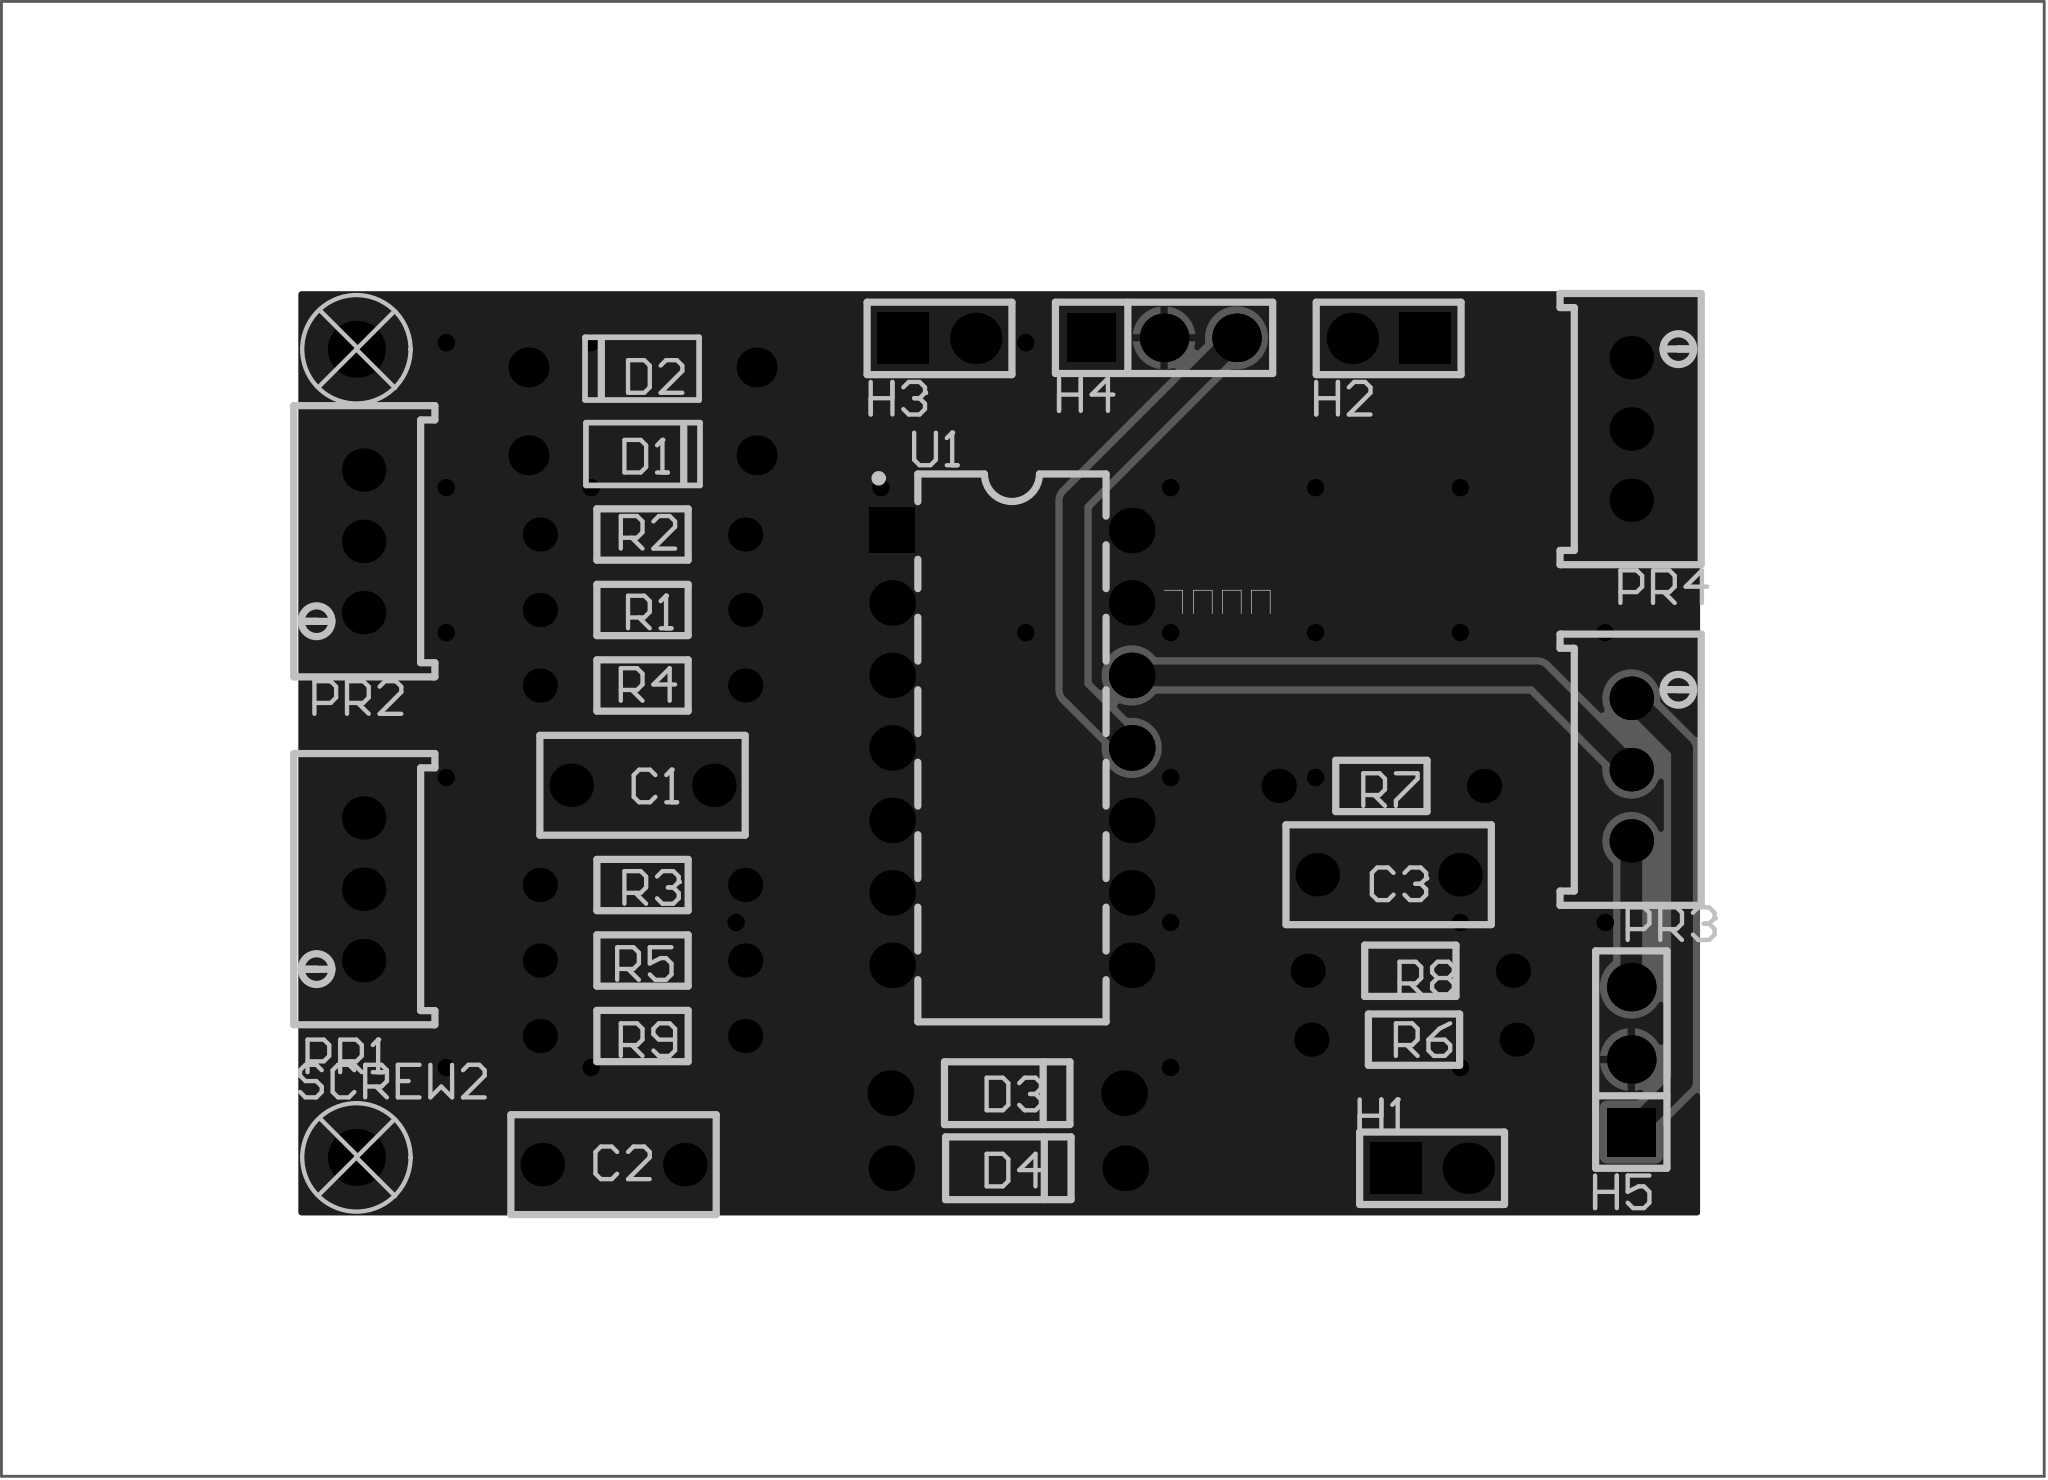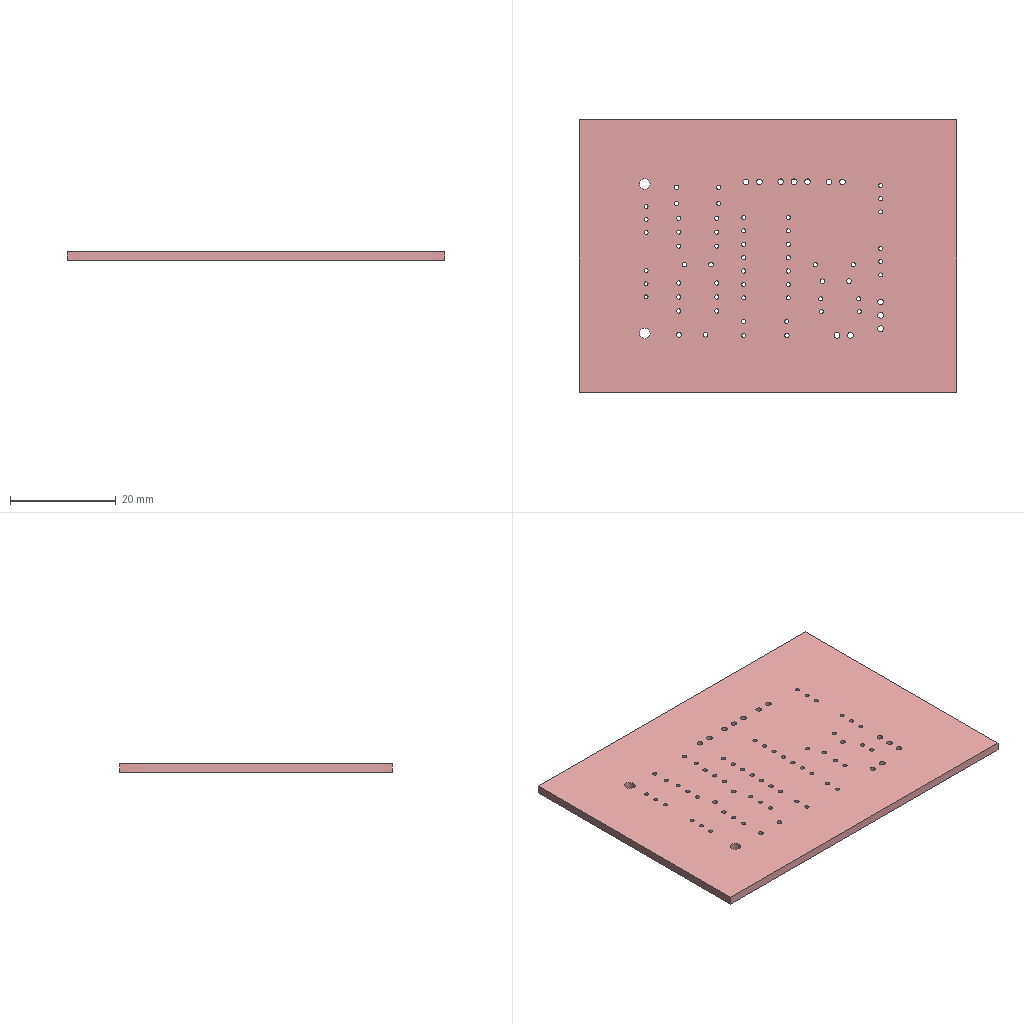Circuit board layout | Altium Designer | box 71.6 x 51.7 x 1.6 mm
Layer stack:
# Altium Designer layer stack of  (unit mm; dielectric type: 0 none, 1 core, 2 prepreg, 3 surface material)
index,name,kind,layer,copper_thickness_mm,dielectric_type,dielectric_thickness_mm,dielectric_material,dielectric_constant
0,Top Paste Mask Layer,other,,,,,,
1,Top Silkscreen Layer,other,,,,,,
2,Top Solder Mask Layer,dielectric,,,3,0.01,,3.3
3,Top Layer,copper,Top Layer,0.035,,,,
4,Dielectric1,dielectric,,,3,1.51,FR4,4.5
5,Bottom Layer,copper,Bottom Layer,0.035,,,,
6,Bottom Solder Mask Layer,dielectric,,,3,0.01,,3.3
7,Bottom Silkscreen Layer,other,,,,,,
8,Bottom Paste Mask Layer,other,,,,,,
# drill layer pairs: low layer,high layer
drill_pair,Top Layer,Bottom Layer
Part placement:
Designator,Comment,Layer,Footprint,Center-X(mm),Center-Y(mm),Rotation
C1,10nF,TopLayer,CAP-TH_L7.2-W3.5-P5.00-D0.6,92.329,94.068,0
C2,10nF,TopLayer,CAP-TH_L7.2-W3.5-P5.00-D0.6,91.313,80.772,0
C3,10nF,TopLayer,CAP-TH_L7.2-W3.5-P5.00-D0.6,118.491,90.932,180
D1,1N4148,TopLayer,DO-35_BD2.2-L4.0-D0.50_1N4148,92.329,105.633,0
D2,1N4148,TopLayer,DO-35_BD2.2-L4.0-D0.50_1N4148,92.329,108.712,180
D3,1.45V,TopLayer,DO-35_BD2.0-L4.2-P8.20-D0.5-RD,105.116,83.276,180
D4,1.45V,TopLayer,DO-35_BD2.0-L4.2-P8.20-D0.5-RD,105.156,80.645,180
H1,,TopLayer,HDR-TH_2P-P2.54-V-M-1,120.015,80.645,0
H2,,TopLayer,HDR-TH_2P-P2.54-V-M-1,118.491,109.728,180
H3,,TopLayer,HDR-TH_2P-P2.54-V-M-1,102.743,109.728,0
PR1,100kΩ,TopLayer,R_3296,82.55,90.424,90
PR2,100kΩ,TopLayer,R_3296,82.55,102.616,90
PR3,1kΩ,TopLayer,R_3296,127,94.615,270
PR4,1kΩ,TopLayer,R_3296,127,106.553,270
R1,10kΩ,TopLayer,Res_1/8W,92.329,100.21,180
R2,10kΩ,TopLayer,Res_1/8W,92.329,102.856,0
R3,790Ω,TopLayer,Res_1/8W,92.329,90.571,180
R4,790Ω,TopLayer,Res_1/8W,92.329,97.565,0
R5,10kΩ,TopLayer,Res_1/8W,92.329,87.926,0
R6,100kΩ,TopLayer,Res_1/8W,119.38,85.153,0
R7,100kΩ,TopLayer,Res_1/8W,118.237,94.044,180
R8,1MΩ,TopLayer,Res_1/8W,119.253,87.567,180
R9,10kΩ,TopLayer,Res_1/8W,92.329,85.28,0
U1,LM324DT,TopLayer,DIP-14_L19.2-W6.6-P2.54-LS10.9-BL,105.283,95.377,270
H4,,TopLayer,HDR-TH_3P-P2.54-V-M,110.617,109.748,0
H5,,TopLayer,HDR-TH_3P-P2.54-V-M,127,84.455,90
SCREW1,,TopLayer,M2螺丝,82.296,109.347,0
SCREW2,,TopLayer,M2螺丝,82.296,81.026,0
Pad and via stacks:
# Altium Designer via and pad stacks of  (unit mm). Each distinct definition once, with the count of objects using it.
# via: kind,start_layer,end_layer,hole_mm,diameter_mm,mode(0 simple;1 top-mid-bottom;2 full stack),diameter_per_layer,count,example_net
# pad: kind,layer,hole_mm,hole_type(0 round;1 square;2 slot),plating,top_size,top_shape(1 round;2 rect;3 octagon;9 rounded rect),mid_size,bottom_size,mode,footprint,size_per_layer,count,example
pad,Multi-Layer,0.9,0,plated,1.524x1.524,1,1.524x1.524,1.524x1.524,0,CAP-TH_L7.2-W3.5-P5.00-D0.6,,6,C1.2
pad,Multi-Layer,0.8,0,plated,1.4x1.4,1,1.4x1.4,1.4x1.4,0,DO-35_BD2.2-L4.0-D0.50_1N4148,,4,D1.2
pad,Multi-Layer,0.8,0,plated,1.6x1.6,1,1.6x1.6,1.6x1.6,0,DO-35_BD2.0-L4.2-P8.20-D0.5-RD,,4,D3.2
pad,Multi-Layer,1.1,0,plated,1.8x1.8,1,1.8x1.8,1.8x1.8,0,HDR-TH_2P-P2.54-V-M-1,,3,H1.2
pad,Multi-Layer,1.1,0,plated,1.8x1.8,2,1.8x1.8,1.8x1.8,0,HDR-TH_2P-P2.54-V-M-1,,3,H1.1
pad,Multi-Layer,0.762,0,plated,1.524x1.524,1,1.524x1.524,1.524x1.524,0,R_3296,,12,PR1.2
pad,Multi-Layer,0.8001,0,plated,1.199x1.199,1,1.199x1.199,1.199x1.199,0,Res_1/8W,,18,R1.1
pad,Multi-Layer,0.8128,0,plated,1.6x1.6,2,1.6x1.6,1.6x1.6,0,DIP-14_L19.2-W6.6-P2.54-LS10.9-BL,,1,U1.1
pad,Multi-Layer,0.8128,0,plated,1.6x1.6,1,1.6x1.6,1.6x1.6,0,DIP-14_L19.2-W6.6-P2.54-LS10.9-BL,,13,U1.2
pad,Multi-Layer,1.1,0,plated,1.7x1.7,2,1.7x1.7,1.7x1.7,0,HDR-TH_3P-P2.54-V-M,,2,H4.1
pad,Multi-Layer,1.1,0,plated,1.7x1.7,1,1.7x1.7,1.7x1.7,0,HDR-TH_3P-P2.54-V-M,,4,H4.2
pad,Multi-Layer,2,0,plated,2x2,1,2x2,2x2,0,M2\u00C2\u00DD\u00CB\u00BF,,2,SCREW1.1
pad,Top Layer,0,0,plated,0.6096x0.6096,1,0.6096x0.6096,0.6096x0.6096,0,,,17,TP1
pad,Bottom Layer,0,0,plated,0.6096x0.6096,1,0.6096x0.6096,0.6096x0.6096,0,,,1,TP16
via,Top Layer,Bottom Layer,0.3048,0.61,0,,26,GND
Copper pours:
name,layer,net,type(0 solid;1 hatched;2 none)
Top Layer-GND,Top Layer,GND,0
Bottom Layer-GND,Bottom Layer,GND,0